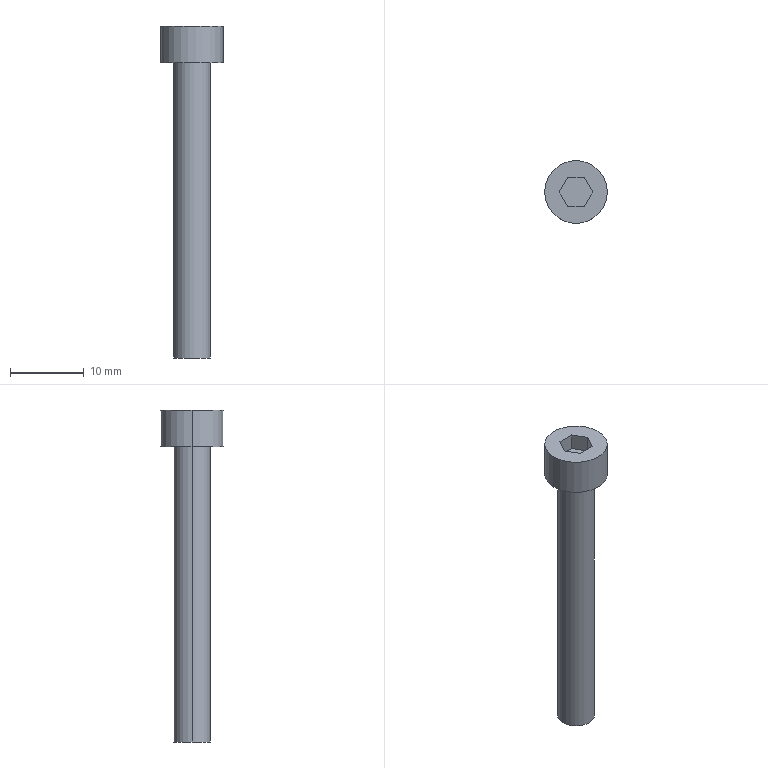Part | SolidWorks | features BaseBody 1 | 1 solid | 14 faces | box 8.5 x 8.5 x 45 mm | volume 1040 mm3 | plane 10 | cylinder 4 | commonest cylinder face diameters 5 x2 8.5 x2
STEP:
#1=CARTESIAN_POINT('',(2.5,0.,-40.));
#2=VERTEX_POINT('',#1);
#3=CARTESIAN_POINT('',(-2.5,0.,-40.));
#4=VERTEX_POINT('',#3);
#5=CARTESIAN_POINT('',(0.,0.,-40.));
#6=DIRECTION('',(0.,0.,1.));
#7=DIRECTION('',(1.,0.,0.));
#8=AXIS2_PLACEMENT_3D('',#5,#6,#7);
#9=CIRCLE('',#8,2.5);
#10=EDGE_CURVE('',#2,#4,#9,.T.);
#11=ORIENTED_EDGE('',*,*,#10,.T.);
#12=CARTESIAN_POINT('',(-2.5,0.,0.));
#13=VERTEX_POINT('',#12);
#14=CARTESIAN_POINT('',(-2.5,0.,-40.));
#15=DIRECTION('',(0.,0.,1.));
#16=VECTOR('',#15,1000.);
#17=LINE('',#14,#16);
#18=EDGE_CURVE('',#4,#13,#17,.T.);
#19=ORIENTED_EDGE('',*,*,#18,.T.);
#20=CARTESIAN_POINT('',(2.5,0.,0.));
#21=VERTEX_POINT('',#20);
#22=CARTESIAN_POINT('',(0.,0.,0.));
#23=DIRECTION('',(0.,0.,-1.));
#24=DIRECTION('',(1.,0.,0.));
#25=AXIS2_PLACEMENT_3D('',#22,#23,#24);
#26=CIRCLE('',#25,2.5);
#27=EDGE_CURVE('',#13,#21,#26,.T.);
#28=ORIENTED_EDGE('',*,*,#27,.T.);
#29=CARTESIAN_POINT('',(2.5,0.,-40.));
#30=DIRECTION('',(0.,0.,1.));
#31=VECTOR('',#30,1000.);
#32=LINE('',#29,#31);
#33=EDGE_CURVE('',#2,#21,#32,.T.);
#34=ORIENTED_EDGE('',*,*,#33,.F.);
#35=EDGE_LOOP('',(#11,#19,#28,#34));
#36=FACE_OUTER_BOUND('',#35,.T.);
#37=CARTESIAN_POINT('',(0.,0.,-40.));
#38=DIRECTION('',(0.,0.,1.));
#39=DIRECTION('',(1.,0.,0.));
#40=AXIS2_PLACEMENT_3D('',#37,#38,#39);
#41=CYLINDRICAL_SURFACE('',#40,2.5);
#42=ADVANCED_FACE('',(#36),#41,.T.);
#43=CARTESIAN_POINT('',(4.25,0.,0.));
#44=VERTEX_POINT('',#43);
#45=CARTESIAN_POINT('',(-4.25,0.,0.));
#46=VERTEX_POINT('',#45);
#47=CARTESIAN_POINT('',(0.,0.,0.));
#48=DIRECTION('',(0.,0.,1.));
#49=DIRECTION('',(1.,0.,0.));
#50=AXIS2_PLACEMENT_3D('',#47,#48,#49);
#51=CIRCLE('',#50,4.25);
#52=EDGE_CURVE('',#44,#46,#51,.T.);
#53=ORIENTED_EDGE('',*,*,#52,.T.);
#54=CARTESIAN_POINT('',(-4.25,0.,5.));
#55=VERTEX_POINT('',#54);
#56=CARTESIAN_POINT('',(-4.25,0.,0.));
#57=DIRECTION('',(0.,0.,1.));
#58=VECTOR('',#57,1000.);
#59=LINE('',#56,#58);
#60=EDGE_CURVE('',#46,#55,#59,.T.);
#61=ORIENTED_EDGE('',*,*,#60,.T.);
#62=CARTESIAN_POINT('',(4.25,0.,5.));
#63=VERTEX_POINT('',#62);
#64=CARTESIAN_POINT('',(0.,0.,5.));
#65=DIRECTION('',(0.,0.,-1.));
#66=DIRECTION('',(1.,0.,0.));
#67=AXIS2_PLACEMENT_3D('',#64,#65,#66);
#68=CIRCLE('',#67,4.25);
#69=EDGE_CURVE('',#55,#63,#68,.T.);
#70=ORIENTED_EDGE('',*,*,#69,.T.);
#71=CARTESIAN_POINT('',(4.25,0.,0.));
#72=DIRECTION('',(0.,0.,1.));
#73=VECTOR('',#72,1000.);
#74=LINE('',#71,#73);
#75=EDGE_CURVE('',#44,#63,#74,.T.);
#76=ORIENTED_EDGE('',*,*,#75,.F.);
#77=EDGE_LOOP('',(#53,#61,#70,#76));
#78=FACE_OUTER_BOUND('',#77,.T.);
#79=CARTESIAN_POINT('',(0.,0.,0.));
#80=DIRECTION('',(0.,0.,1.));
#81=DIRECTION('',(1.,0.,0.));
#82=AXIS2_PLACEMENT_3D('',#79,#80,#81);
#83=CYLINDRICAL_SURFACE('',#82,4.25);
#84=ADVANCED_FACE('',(#78),#83,.T.);
#85=ORIENTED_EDGE('',*,*,#18,.F.);
#86=CARTESIAN_POINT('',(0.,0.,-40.));
#87=DIRECTION('',(0.,0.,1.));
#88=DIRECTION('',(1.,0.,0.));
#89=AXIS2_PLACEMENT_3D('',#86,#87,#88);
#90=CIRCLE('',#89,2.5);
#91=EDGE_CURVE('',#4,#2,#90,.T.);
#92=ORIENTED_EDGE('',*,*,#91,.T.);
#93=ORIENTED_EDGE('',*,*,#33,.T.);
#94=CARTESIAN_POINT('',(0.,0.,0.));
#95=DIRECTION('',(0.,0.,-1.));
#96=DIRECTION('',(1.,0.,0.));
#97=AXIS2_PLACEMENT_3D('',#94,#95,#96);
#98=CIRCLE('',#97,2.5);
#99=EDGE_CURVE('',#21,#13,#98,.T.);
#100=ORIENTED_EDGE('',*,*,#99,.T.);
#101=EDGE_LOOP('',(#85,#92,#93,#100));
#102=FACE_OUTER_BOUND('',#101,.T.);
#103=CARTESIAN_POINT('',(0.,0.,-40.));
#104=DIRECTION('',(0.,0.,1.));
#105=DIRECTION('',(1.,0.,0.));
#106=AXIS2_PLACEMENT_3D('',#103,#104,#105);
#107=CYLINDRICAL_SURFACE('',#106,2.5);
#108=ADVANCED_FACE('',(#102),#107,.T.);
#109=ORIENTED_EDGE('',*,*,#10,.F.);
#110=ORIENTED_EDGE('',*,*,#91,.F.);
#111=EDGE_LOOP('',(#109,#110));
#112=FACE_OUTER_BOUND('',#111,.T.);
#113=CARTESIAN_POINT('',(0.,0.,-40.));
#114=DIRECTION('',(0.,0.,1.));
#115=DIRECTION('',(1.,0.,0.));
#116=AXIS2_PLACEMENT_3D('',#113,#114,#115);
#117=PLANE('',#116);
#118=ADVANCED_FACE('',(#112),#117,.F.);
#119=ORIENTED_EDGE('',*,*,#99,.F.);
#120=ORIENTED_EDGE('',*,*,#27,.F.);
#121=EDGE_LOOP('',(#119,#120));
#122=FACE_BOUND('',#121,.T.);
#123=ORIENTED_EDGE('',*,*,#52,.F.);
#124=CARTESIAN_POINT('',(0.,0.,0.));
#125=DIRECTION('',(0.,0.,1.));
#126=DIRECTION('',(1.,0.,0.));
#127=AXIS2_PLACEMENT_3D('',#124,#125,#126);
#128=CIRCLE('',#127,4.25);
#129=EDGE_CURVE('',#46,#44,#128,.T.);
#130=ORIENTED_EDGE('',*,*,#129,.F.);
#131=EDGE_LOOP('',(#123,#130));
#132=FACE_OUTER_BOUND('',#131,.T.);
#133=CARTESIAN_POINT('',(0.,0.,0.));
#134=DIRECTION('',(0.,0.,1.));
#135=DIRECTION('',(1.,0.,0.));
#136=AXIS2_PLACEMENT_3D('',#133,#134,#135);
#137=PLANE('',#136);
#138=ADVANCED_FACE('',(#122,#132),#137,.F.);
#139=ORIENTED_EDGE('',*,*,#60,.F.);
#140=ORIENTED_EDGE('',*,*,#129,.T.);
#141=ORIENTED_EDGE('',*,*,#75,.T.);
#142=CARTESIAN_POINT('',(0.,0.,5.));
#143=DIRECTION('',(0.,0.,-1.));
#144=DIRECTION('',(1.,0.,0.));
#145=AXIS2_PLACEMENT_3D('',#142,#143,#144);
#146=CIRCLE('',#145,4.25);
#147=EDGE_CURVE('',#63,#55,#146,.T.);
#148=ORIENTED_EDGE('',*,*,#147,.T.);
#149=EDGE_LOOP('',(#139,#140,#141,#148));
#150=FACE_OUTER_BOUND('',#149,.T.);
#151=CARTESIAN_POINT('',(0.,0.,0.));
#152=DIRECTION('',(0.,0.,1.));
#153=DIRECTION('',(1.,0.,0.));
#154=AXIS2_PLACEMENT_3D('',#151,#152,#153);
#155=CYLINDRICAL_SURFACE('',#154,4.25);
#156=ADVANCED_FACE('',(#150),#155,.T.);
#157=CARTESIAN_POINT('',(-1.125,-1.949,5.));
#158=VERTEX_POINT('',#157);
#159=CARTESIAN_POINT('',(-2.25,0.,5.));
#160=VERTEX_POINT('',#159);
#161=CARTESIAN_POINT('',(-1.125,-1.949,5.));
#162=DIRECTION('',(-0.5,0.866,0.));
#163=VECTOR('',#162,1000.);
#164=LINE('',#161,#163);
#165=EDGE_CURVE('',#158,#160,#164,.T.);
#166=ORIENTED_EDGE('',*,*,#165,.T.);
#167=CARTESIAN_POINT('',(-1.125,1.949,5.));
#168=VERTEX_POINT('',#167);
#169=CARTESIAN_POINT('',(-2.25,0.,5.));
#170=DIRECTION('',(0.5,0.866,0.));
#171=VECTOR('',#170,1000.);
#172=LINE('',#169,#171);
#173=EDGE_CURVE('',#160,#168,#172,.T.);
#174=ORIENTED_EDGE('',*,*,#173,.T.);
#175=CARTESIAN_POINT('',(1.125,1.949,5.));
#176=VERTEX_POINT('',#175);
#177=CARTESIAN_POINT('',(0.,1.949,5.));
#178=DIRECTION('',(1.,0.,0.));
#179=VECTOR('',#178,1000.);
#180=LINE('',#177,#179);
#181=EDGE_CURVE('',#168,#176,#180,.T.);
#182=ORIENTED_EDGE('',*,*,#181,.T.);
#183=CARTESIAN_POINT('',(2.25,0.,5.));
#184=VERTEX_POINT('',#183);
#185=CARTESIAN_POINT('',(1.125,1.949,5.));
#186=DIRECTION('',(0.5,-0.866,0.));
#187=VECTOR('',#186,1000.);
#188=LINE('',#185,#187);
#189=EDGE_CURVE('',#176,#184,#188,.T.);
#190=ORIENTED_EDGE('',*,*,#189,.T.);
#191=CARTESIAN_POINT('',(1.125,-1.949,5.));
#192=VERTEX_POINT('',#191);
#193=CARTESIAN_POINT('',(2.25,0.,5.));
#194=DIRECTION('',(-0.5,-0.866,0.));
#195=VECTOR('',#194,1000.);
#196=LINE('',#193,#195);
#197=EDGE_CURVE('',#184,#192,#196,.T.);
#198=ORIENTED_EDGE('',*,*,#197,.T.);
#199=CARTESIAN_POINT('',(0.,-1.949,5.));
#200=DIRECTION('',(-1.,0.,0.));
#201=VECTOR('',#200,1000.);
#202=LINE('',#199,#201);
#203=EDGE_CURVE('',#192,#158,#202,.T.);
#204=ORIENTED_EDGE('',*,*,#203,.T.);
#205=EDGE_LOOP('',(#166,#174,#182,#190,#198,#204));
#206=FACE_BOUND('',#205,.T.);
#207=ORIENTED_EDGE('',*,*,#147,.F.);
#208=ORIENTED_EDGE('',*,*,#69,.F.);
#209=EDGE_LOOP('',(#207,#208));
#210=FACE_OUTER_BOUND('',#209,.T.);
#211=CARTESIAN_POINT('',(0.,0.,5.));
#212=DIRECTION('',(0.,0.,1.));
#213=DIRECTION('',(1.,0.,0.));
#214=AXIS2_PLACEMENT_3D('',#211,#212,#213);
#215=PLANE('',#214);
#216=ADVANCED_FACE('',(#206,#210),#215,.T.);
#217=ORIENTED_EDGE('',*,*,#173,.F.);
#218=CARTESIAN_POINT('',(-2.25,0.,2.75));
#219=VERTEX_POINT('',#218);
#220=CARTESIAN_POINT('',(-2.25,0.,2.75));
#221=DIRECTION('',(0.,0.,-1.));
#222=VECTOR('',#221,1000.);
#223=LINE('',#220,#222);
#224=EDGE_CURVE('',#160,#219,#223,.T.);
#225=ORIENTED_EDGE('',*,*,#224,.T.);
#226=CARTESIAN_POINT('',(-1.125,1.949,2.75));
#227=VERTEX_POINT('',#226);
#228=CARTESIAN_POINT('',(-1.125,1.949,2.75));
#229=DIRECTION('',(0.5,0.866,0.));
#230=VECTOR('',#229,1000.);
#231=LINE('',#228,#230);
#232=EDGE_CURVE('',#219,#227,#231,.T.);
#233=ORIENTED_EDGE('',*,*,#232,.T.);
#234=CARTESIAN_POINT('',(-1.125,1.949,2.75));
#235=DIRECTION('',(0.,0.,1.));
#236=VECTOR('',#235,1000.);
#237=LINE('',#234,#236);
#238=EDGE_CURVE('',#227,#168,#237,.T.);
#239=ORIENTED_EDGE('',*,*,#238,.T.);
#240=EDGE_LOOP('',(#217,#225,#233,#239));
#241=FACE_OUTER_BOUND('',#240,.T.);
#242=CARTESIAN_POINT('',(-1.125,1.949,2.75));
#243=DIRECTION('',(0.866,-0.5,0.));
#244=DIRECTION('',(0.5,0.866,0.));
#245=AXIS2_PLACEMENT_3D('',#242,#243,#244);
#246=PLANE('',#245);
#247=ADVANCED_FACE('',(#241),#246,.T.);
#248=ORIENTED_EDGE('',*,*,#165,.F.);
#249=CARTESIAN_POINT('',(-1.125,-1.949,2.75));
#250=VERTEX_POINT('',#249);
#251=CARTESIAN_POINT('',(-1.125,-1.949,2.75));
#252=DIRECTION('',(0.,0.,-1.));
#253=VECTOR('',#252,1000.);
#254=LINE('',#251,#253);
#255=EDGE_CURVE('',#158,#250,#254,.T.);
#256=ORIENTED_EDGE('',*,*,#255,.T.);
#257=CARTESIAN_POINT('',(-2.25,0.,2.75));
#258=DIRECTION('',(-0.5,0.866,0.));
#259=VECTOR('',#258,1000.);
#260=LINE('',#257,#259);
#261=EDGE_CURVE('',#250,#219,#260,.T.);
#262=ORIENTED_EDGE('',*,*,#261,.T.);
#263=ORIENTED_EDGE('',*,*,#224,.F.);
#264=EDGE_LOOP('',(#248,#256,#262,#263));
#265=FACE_OUTER_BOUND('',#264,.T.);
#266=CARTESIAN_POINT('',(-2.25,0.,2.75));
#267=DIRECTION('',(0.866,0.5,0.));
#268=DIRECTION('',(-0.5,0.866,0.));
#269=AXIS2_PLACEMENT_3D('',#266,#267,#268);
#270=PLANE('',#269);
#271=ADVANCED_FACE('',(#265),#270,.T.);
#272=ORIENTED_EDGE('',*,*,#203,.F.);
#273=CARTESIAN_POINT('',(1.125,-1.949,2.75));
#274=VERTEX_POINT('',#273);
#275=CARTESIAN_POINT('',(1.125,-1.949,2.75));
#276=DIRECTION('',(0.,0.,-1.));
#277=VECTOR('',#276,1000.);
#278=LINE('',#275,#277);
#279=EDGE_CURVE('',#192,#274,#278,.T.);
#280=ORIENTED_EDGE('',*,*,#279,.T.);
#281=CARTESIAN_POINT('',(-1.125,-1.949,2.75));
#282=DIRECTION('',(-1.,0.,0.));
#283=VECTOR('',#282,1000.);
#284=LINE('',#281,#283);
#285=EDGE_CURVE('',#274,#250,#284,.T.);
#286=ORIENTED_EDGE('',*,*,#285,.T.);
#287=ORIENTED_EDGE('',*,*,#255,.F.);
#288=EDGE_LOOP('',(#272,#280,#286,#287));
#289=FACE_OUTER_BOUND('',#288,.T.);
#290=CARTESIAN_POINT('',(-1.125,-1.949,2.75));
#291=DIRECTION('',(0.,1.,0.));
#292=DIRECTION('',(-1.,0.,0.));
#293=AXIS2_PLACEMENT_3D('',#290,#291,#292);
#294=PLANE('',#293);
#295=ADVANCED_FACE('',(#289),#294,.T.);
#296=ORIENTED_EDGE('',*,*,#197,.F.);
#297=CARTESIAN_POINT('',(2.25,0.,2.75));
#298=VERTEX_POINT('',#297);
#299=CARTESIAN_POINT('',(2.25,0.,2.75));
#300=DIRECTION('',(0.,0.,-1.));
#301=VECTOR('',#300,1000.);
#302=LINE('',#299,#301);
#303=EDGE_CURVE('',#184,#298,#302,.T.);
#304=ORIENTED_EDGE('',*,*,#303,.T.);
#305=CARTESIAN_POINT('',(1.125,-1.949,2.75));
#306=DIRECTION('',(-0.5,-0.866,0.));
#307=VECTOR('',#306,1000.);
#308=LINE('',#305,#307);
#309=EDGE_CURVE('',#298,#274,#308,.T.);
#310=ORIENTED_EDGE('',*,*,#309,.T.);
#311=ORIENTED_EDGE('',*,*,#279,.F.);
#312=EDGE_LOOP('',(#296,#304,#310,#311));
#313=FACE_OUTER_BOUND('',#312,.T.);
#314=CARTESIAN_POINT('',(1.125,-1.949,2.75));
#315=DIRECTION('',(-0.866,0.5,0.));
#316=DIRECTION('',(-0.5,-0.866,0.));
#317=AXIS2_PLACEMENT_3D('',#314,#315,#316);
#318=PLANE('',#317);
#319=ADVANCED_FACE('',(#313),#318,.T.);
#320=ORIENTED_EDGE('',*,*,#189,.F.);
#321=CARTESIAN_POINT('',(1.125,1.949,2.75));
#322=VERTEX_POINT('',#321);
#323=CARTESIAN_POINT('',(1.125,1.949,2.75));
#324=DIRECTION('',(0.,0.,-1.));
#325=VECTOR('',#324,1000.);
#326=LINE('',#323,#325);
#327=EDGE_CURVE('',#176,#322,#326,.T.);
#328=ORIENTED_EDGE('',*,*,#327,.T.);
#329=CARTESIAN_POINT('',(2.25,0.,2.75));
#330=DIRECTION('',(0.5,-0.866,0.));
#331=VECTOR('',#330,1000.);
#332=LINE('',#329,#331);
#333=EDGE_CURVE('',#322,#298,#332,.T.);
#334=ORIENTED_EDGE('',*,*,#333,.T.);
#335=ORIENTED_EDGE('',*,*,#303,.F.);
#336=EDGE_LOOP('',(#320,#328,#334,#335));
#337=FACE_OUTER_BOUND('',#336,.T.);
#338=CARTESIAN_POINT('',(2.25,0.,2.75));
#339=DIRECTION('',(-0.866,-0.5,0.));
#340=DIRECTION('',(0.5,-0.866,0.));
#341=AXIS2_PLACEMENT_3D('',#338,#339,#340);
#342=PLANE('',#341);
#343=ADVANCED_FACE('',(#337),#342,.T.);
#344=ORIENTED_EDGE('',*,*,#181,.F.);
#345=ORIENTED_EDGE('',*,*,#238,.F.);
#346=CARTESIAN_POINT('',(1.125,1.949,2.75));
#347=DIRECTION('',(1.,0.,0.));
#348=VECTOR('',#347,1000.);
#349=LINE('',#346,#348);
#350=EDGE_CURVE('',#227,#322,#349,.T.);
#351=ORIENTED_EDGE('',*,*,#350,.T.);
#352=ORIENTED_EDGE('',*,*,#327,.F.);
#353=EDGE_LOOP('',(#344,#345,#351,#352));
#354=FACE_OUTER_BOUND('',#353,.T.);
#355=CARTESIAN_POINT('',(1.125,1.949,2.75));
#356=DIRECTION('',(0.,-1.,0.));
#357=DIRECTION('',(1.,0.,0.));
#358=AXIS2_PLACEMENT_3D('',#355,#356,#357);
#359=PLANE('',#358);
#360=ADVANCED_FACE('',(#354),#359,.T.);
#361=ORIENTED_EDGE('',*,*,#285,.F.);
#362=ORIENTED_EDGE('',*,*,#309,.F.);
#363=ORIENTED_EDGE('',*,*,#333,.F.);
#364=ORIENTED_EDGE('',*,*,#350,.F.);
#365=ORIENTED_EDGE('',*,*,#232,.F.);
#366=ORIENTED_EDGE('',*,*,#261,.F.);
#367=EDGE_LOOP('',(#361,#362,#363,#364,#365,#366));
#368=FACE_OUTER_BOUND('',#367,.T.);
#369=CARTESIAN_POINT('',(0.,0.,2.75));
#370=DIRECTION('',(0.,0.,1.));
#371=DIRECTION('',(1.,0.,0.));
#372=AXIS2_PLACEMENT_3D('',#369,#370,#371);
#373=PLANE('',#372);
#374=ADVANCED_FACE('',(#368),#373,.T.);
#375=CLOSED_SHELL('',(#42,#84,#108,#118,#138,#156,#216,#247,#271,#295,#319,#343,#360,#374));
#376=MANIFOLD_SOLID_BREP('',#375);
#377=CARTESIAN_POINT('',(0.,0.,0.));
#378=DIRECTION('',(0.,0.,1.));
#379=DIRECTION('',(1.,0.,0.));
#380=AXIS2_PLACEMENT_3D('',#377,#378,#379);
#381=(LENGTH_UNIT()NAMED_UNIT(*)SI_UNIT(.MILLI.,.METRE.));
#382=UNCERTAINTY_MEASURE_WITH_UNIT(LENGTH_MEASURE(0.00001),#381,'','');
#383=(NAMED_UNIT(*)PLANE_ANGLE_UNIT()SI_UNIT($,.RADIAN.));
#384=(NAMED_UNIT(*)SI_UNIT($,.STERADIAN.)SOLID_ANGLE_UNIT());
#385=(GEOMETRIC_REPRESENTATION_CONTEXT(3)GLOBAL_UNCERTAINTY_ASSIGNED_CONTEXT((#382))GLOBAL_UNIT_ASSIGNED_CONTEXT((#381,#383,#384))REPRESENTATION_CONTEXT('',''));
#386=ADVANCED_BREP_SHAPE_REPRESENTATION('',(#376,#380),#385);